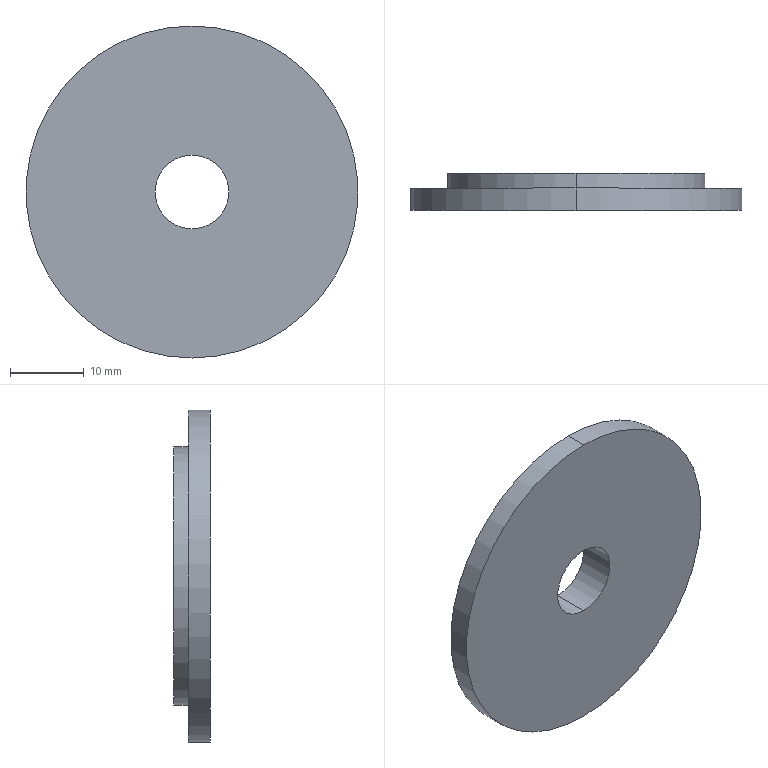Part | SolidWorks | features ICE 2, Extrusion 1 | 1 solid | 9 faces | box 45 x 5 x 45 mm | volume 6303 mm3 | cylinder 6 | plane 3 | commonest cylinder face diameters 10 x2 35 x2 45 x2
STEP:
#1=CARTESIAN_POINT('',(0.,0.,-5.));
#2=VERTEX_POINT('',#1);
#3=CARTESIAN_POINT('',(0.,0.,5.));
#4=VERTEX_POINT('',#3);
#5=CARTESIAN_POINT('',(0.,0.,0.));
#6=DIRECTION('',(0.,1.,0.));
#7=DIRECTION('',(0.,0.,1.));
#8=AXIS2_PLACEMENT_3D('',#5,#6,#7);
#9=CIRCLE('',#8,5.);
#10=EDGE_CURVE('',#2,#4,#9,.T.);
#11=ORIENTED_EDGE('',*,*,#10,.F.);
#12=CARTESIAN_POINT('',(0.,5.,-5.));
#13=VERTEX_POINT('',#12);
#14=CARTESIAN_POINT('',(0.,0.,-5.));
#15=DIRECTION('',(0.,1.,0.));
#16=VECTOR('',#15,1000.);
#17=LINE('',#14,#16);
#18=EDGE_CURVE('',#2,#13,#17,.T.);
#19=ORIENTED_EDGE('',*,*,#18,.T.);
#20=CARTESIAN_POINT('',(0.,5.,5.));
#21=VERTEX_POINT('',#20);
#22=CARTESIAN_POINT('',(0.,5.,0.));
#23=DIRECTION('',(0.,1.,0.));
#24=DIRECTION('',(0.,0.,1.));
#25=AXIS2_PLACEMENT_3D('',#22,#23,#24);
#26=CIRCLE('',#25,5.);
#27=EDGE_CURVE('',#13,#21,#26,.T.);
#28=ORIENTED_EDGE('',*,*,#27,.T.);
#29=CARTESIAN_POINT('',(0.,0.,5.));
#30=DIRECTION('',(0.,1.,0.));
#31=VECTOR('',#30,1000.);
#32=LINE('',#29,#31);
#33=EDGE_CURVE('',#4,#21,#32,.T.);
#34=ORIENTED_EDGE('',*,*,#33,.F.);
#35=EDGE_LOOP('',(#11,#19,#28,#34));
#36=FACE_OUTER_BOUND('',#35,.T.);
#37=CARTESIAN_POINT('',(0.,0.,0.));
#38=DIRECTION('',(0.,1.,0.));
#39=DIRECTION('',(0.,0.,1.));
#40=AXIS2_PLACEMENT_3D('',#37,#38,#39);
#41=CYLINDRICAL_SURFACE('',#40,5.);
#42=ADVANCED_FACE('',(#36),#41,.F.);
#43=CARTESIAN_POINT('',(0.,5.,17.5));
#44=VERTEX_POINT('',#43);
#45=CARTESIAN_POINT('',(0.,5.,-17.5));
#46=VERTEX_POINT('',#45);
#47=CARTESIAN_POINT('',(0.,5.,0.));
#48=DIRECTION('',(0.,1.,0.));
#49=DIRECTION('',(0.,0.,1.));
#50=AXIS2_PLACEMENT_3D('',#47,#48,#49);
#51=CIRCLE('',#50,17.5);
#52=EDGE_CURVE('',#44,#46,#51,.T.);
#53=ORIENTED_EDGE('',*,*,#52,.F.);
#54=CARTESIAN_POINT('',(0.,3.,17.5));
#55=VERTEX_POINT('',#54);
#56=CARTESIAN_POINT('',(0.,5.,17.5));
#57=DIRECTION('',(0.,-1.,0.));
#58=VECTOR('',#57,1000.);
#59=LINE('',#56,#58);
#60=EDGE_CURVE('',#44,#55,#59,.T.);
#61=ORIENTED_EDGE('',*,*,#60,.T.);
#62=CARTESIAN_POINT('',(0.,3.,-17.5));
#63=VERTEX_POINT('',#62);
#64=CARTESIAN_POINT('',(0.,3.,0.));
#65=DIRECTION('',(0.,1.,0.));
#66=DIRECTION('',(0.,0.,1.));
#67=AXIS2_PLACEMENT_3D('',#64,#65,#66);
#68=CIRCLE('',#67,17.5);
#69=EDGE_CURVE('',#55,#63,#68,.T.);
#70=ORIENTED_EDGE('',*,*,#69,.T.);
#71=CARTESIAN_POINT('',(0.,5.,-17.5));
#72=DIRECTION('',(0.,-1.,0.));
#73=VECTOR('',#72,1000.);
#74=LINE('',#71,#73);
#75=EDGE_CURVE('',#46,#63,#74,.T.);
#76=ORIENTED_EDGE('',*,*,#75,.F.);
#77=EDGE_LOOP('',(#53,#61,#70,#76));
#78=FACE_OUTER_BOUND('',#77,.T.);
#79=CARTESIAN_POINT('',(0.,5.,0.));
#80=DIRECTION('',(0.,-1.,0.));
#81=DIRECTION('',(0.,0.,-1.));
#82=AXIS2_PLACEMENT_3D('',#79,#80,#81);
#83=CYLINDRICAL_SURFACE('',#82,17.5);
#84=ADVANCED_FACE('',(#78),#83,.T.);
#85=CARTESIAN_POINT('',(0.,3.,22.5));
#86=VERTEX_POINT('',#85);
#87=CARTESIAN_POINT('',(0.,3.,-22.5));
#88=VERTEX_POINT('',#87);
#89=CARTESIAN_POINT('',(0.,3.,0.));
#90=DIRECTION('',(0.,1.,0.));
#91=DIRECTION('',(0.,0.,1.));
#92=AXIS2_PLACEMENT_3D('',#89,#90,#91);
#93=CIRCLE('',#92,22.5);
#94=EDGE_CURVE('',#86,#88,#93,.T.);
#95=ORIENTED_EDGE('',*,*,#94,.F.);
#96=CARTESIAN_POINT('',(0.,0.,22.5));
#97=VERTEX_POINT('',#96);
#98=CARTESIAN_POINT('',(0.,3.,22.5));
#99=DIRECTION('',(0.,-1.,0.));
#100=VECTOR('',#99,1000.);
#101=LINE('',#98,#100);
#102=EDGE_CURVE('',#86,#97,#101,.T.);
#103=ORIENTED_EDGE('',*,*,#102,.T.);
#104=CARTESIAN_POINT('',(0.,0.,-22.5));
#105=VERTEX_POINT('',#104);
#106=CARTESIAN_POINT('',(0.,0.,0.));
#107=DIRECTION('',(0.,1.,0.));
#108=DIRECTION('',(0.,0.,1.));
#109=AXIS2_PLACEMENT_3D('',#106,#107,#108);
#110=CIRCLE('',#109,22.5);
#111=EDGE_CURVE('',#97,#105,#110,.T.);
#112=ORIENTED_EDGE('',*,*,#111,.T.);
#113=CARTESIAN_POINT('',(0.,3.,-22.5));
#114=DIRECTION('',(0.,-1.,0.));
#115=VECTOR('',#114,1000.);
#116=LINE('',#113,#115);
#117=EDGE_CURVE('',#88,#105,#116,.T.);
#118=ORIENTED_EDGE('',*,*,#117,.F.);
#119=EDGE_LOOP('',(#95,#103,#112,#118));
#120=FACE_OUTER_BOUND('',#119,.T.);
#121=CARTESIAN_POINT('',(0.,3.,0.));
#122=DIRECTION('',(0.,-1.,0.));
#123=DIRECTION('',(0.,0.,-1.));
#124=AXIS2_PLACEMENT_3D('',#121,#122,#123);
#125=CYLINDRICAL_SURFACE('',#124,22.5);
#126=ADVANCED_FACE('',(#120),#125,.T.);
#127=CARTESIAN_POINT('',(0.,3.,0.));
#128=DIRECTION('',(0.,1.,0.));
#129=DIRECTION('',(0.,0.,1.));
#130=AXIS2_PLACEMENT_3D('',#127,#128,#129);
#131=CIRCLE('',#130,22.5);
#132=EDGE_CURVE('',#88,#86,#131,.T.);
#133=ORIENTED_EDGE('',*,*,#132,.T.);
#134=ORIENTED_EDGE('',*,*,#94,.T.);
#135=EDGE_LOOP('',(#133,#134));
#136=FACE_OUTER_BOUND('',#135,.T.);
#137=CARTESIAN_POINT('',(0.,3.,0.));
#138=DIRECTION('',(0.,1.,0.));
#139=DIRECTION('',(0.,0.,1.));
#140=AXIS2_PLACEMENT_3D('',#137,#138,#139);
#141=CIRCLE('',#140,17.5);
#142=EDGE_CURVE('',#63,#55,#141,.T.);
#143=ORIENTED_EDGE('',*,*,#142,.F.);
#144=ORIENTED_EDGE('',*,*,#69,.F.);
#145=EDGE_LOOP('',(#143,#144));
#146=FACE_BOUND('',#145,.T.);
#147=CARTESIAN_POINT('',(0.,3.,0.));
#148=DIRECTION('',(0.,1.,0.));
#149=DIRECTION('',(0.,0.,1.));
#150=AXIS2_PLACEMENT_3D('',#147,#148,#149);
#151=PLANE('',#150);
#152=ADVANCED_FACE('',(#136,#146),#151,.T.);
#153=ORIENTED_EDGE('',*,*,#102,.F.);
#154=ORIENTED_EDGE('',*,*,#132,.F.);
#155=ORIENTED_EDGE('',*,*,#117,.T.);
#156=CARTESIAN_POINT('',(0.,0.,0.));
#157=DIRECTION('',(0.,1.,0.));
#158=DIRECTION('',(0.,0.,1.));
#159=AXIS2_PLACEMENT_3D('',#156,#157,#158);
#160=CIRCLE('',#159,22.5);
#161=EDGE_CURVE('',#105,#97,#160,.T.);
#162=ORIENTED_EDGE('',*,*,#161,.T.);
#163=EDGE_LOOP('',(#153,#154,#155,#162));
#164=FACE_OUTER_BOUND('',#163,.T.);
#165=CARTESIAN_POINT('',(0.,3.,0.));
#166=DIRECTION('',(0.,-1.,0.));
#167=DIRECTION('',(0.,0.,-1.));
#168=AXIS2_PLACEMENT_3D('',#165,#166,#167);
#169=CYLINDRICAL_SURFACE('',#168,22.5);
#170=ADVANCED_FACE('',(#164),#169,.T.);
#171=CARTESIAN_POINT('',(0.,0.,0.));
#172=DIRECTION('',(0.,1.,0.));
#173=DIRECTION('',(0.,0.,1.));
#174=AXIS2_PLACEMENT_3D('',#171,#172,#173);
#175=CIRCLE('',#174,5.);
#176=EDGE_CURVE('',#4,#2,#175,.T.);
#177=ORIENTED_EDGE('',*,*,#176,.T.);
#178=ORIENTED_EDGE('',*,*,#10,.T.);
#179=EDGE_LOOP('',(#177,#178));
#180=FACE_BOUND('',#179,.T.);
#181=ORIENTED_EDGE('',*,*,#161,.F.);
#182=ORIENTED_EDGE('',*,*,#111,.F.);
#183=EDGE_LOOP('',(#181,#182));
#184=FACE_OUTER_BOUND('',#183,.T.);
#185=CARTESIAN_POINT('',(0.,0.,0.));
#186=DIRECTION('',(0.,1.,0.));
#187=DIRECTION('',(0.,0.,1.));
#188=AXIS2_PLACEMENT_3D('',#185,#186,#187);
#189=PLANE('',#188);
#190=ADVANCED_FACE('',(#180,#184),#189,.F.);
#191=ORIENTED_EDGE('',*,*,#60,.F.);
#192=CARTESIAN_POINT('',(0.,5.,0.));
#193=DIRECTION('',(0.,1.,0.));
#194=DIRECTION('',(0.,0.,1.));
#195=AXIS2_PLACEMENT_3D('',#192,#193,#194);
#196=CIRCLE('',#195,17.5);
#197=EDGE_CURVE('',#46,#44,#196,.T.);
#198=ORIENTED_EDGE('',*,*,#197,.F.);
#199=ORIENTED_EDGE('',*,*,#75,.T.);
#200=ORIENTED_EDGE('',*,*,#142,.T.);
#201=EDGE_LOOP('',(#191,#198,#199,#200));
#202=FACE_OUTER_BOUND('',#201,.T.);
#203=CARTESIAN_POINT('',(0.,5.,0.));
#204=DIRECTION('',(0.,-1.,0.));
#205=DIRECTION('',(0.,0.,-1.));
#206=AXIS2_PLACEMENT_3D('',#203,#204,#205);
#207=CYLINDRICAL_SURFACE('',#206,17.5);
#208=ADVANCED_FACE('',(#202),#207,.T.);
#209=CARTESIAN_POINT('',(0.,5.,0.));
#210=DIRECTION('',(0.,1.,0.));
#211=DIRECTION('',(0.,0.,1.));
#212=AXIS2_PLACEMENT_3D('',#209,#210,#211);
#213=CIRCLE('',#212,5.);
#214=EDGE_CURVE('',#21,#13,#213,.T.);
#215=ORIENTED_EDGE('',*,*,#214,.F.);
#216=ORIENTED_EDGE('',*,*,#27,.F.);
#217=EDGE_LOOP('',(#215,#216));
#218=FACE_BOUND('',#217,.T.);
#219=ORIENTED_EDGE('',*,*,#197,.T.);
#220=ORIENTED_EDGE('',*,*,#52,.T.);
#221=EDGE_LOOP('',(#219,#220));
#222=FACE_OUTER_BOUND('',#221,.T.);
#223=CARTESIAN_POINT('',(0.,5.,0.));
#224=DIRECTION('',(0.,1.,0.));
#225=DIRECTION('',(0.,0.,1.));
#226=AXIS2_PLACEMENT_3D('',#223,#224,#225);
#227=PLANE('',#226);
#228=ADVANCED_FACE('',(#218,#222),#227,.T.);
#229=ORIENTED_EDGE('',*,*,#18,.F.);
#230=ORIENTED_EDGE('',*,*,#176,.F.);
#231=ORIENTED_EDGE('',*,*,#33,.T.);
#232=ORIENTED_EDGE('',*,*,#214,.T.);
#233=EDGE_LOOP('',(#229,#230,#231,#232));
#234=FACE_OUTER_BOUND('',#233,.T.);
#235=CARTESIAN_POINT('',(0.,0.,0.));
#236=DIRECTION('',(0.,1.,0.));
#237=DIRECTION('',(0.,0.,1.));
#238=AXIS2_PLACEMENT_3D('',#235,#236,#237);
#239=CYLINDRICAL_SURFACE('',#238,5.);
#240=ADVANCED_FACE('',(#234),#239,.F.);
#241=CLOSED_SHELL('',(#42,#84,#126,#152,#170,#190,#208,#228,#240));
#242=MANIFOLD_SOLID_BREP('',#241);
#243=CARTESIAN_POINT('',(0.,0.,0.));
#244=DIRECTION('',(0.,0.,1.));
#245=DIRECTION('',(1.,0.,0.));
#246=AXIS2_PLACEMENT_3D('',#243,#244,#245);
#247=(LENGTH_UNIT()NAMED_UNIT(*)SI_UNIT(.MILLI.,.METRE.));
#248=UNCERTAINTY_MEASURE_WITH_UNIT(LENGTH_MEASURE(0.00001),#247,'','');
#249=(NAMED_UNIT(*)PLANE_ANGLE_UNIT()SI_UNIT($,.RADIAN.));
#250=(NAMED_UNIT(*)SI_UNIT($,.STERADIAN.)SOLID_ANGLE_UNIT());
#251=(GEOMETRIC_REPRESENTATION_CONTEXT(3)GLOBAL_UNCERTAINTY_ASSIGNED_CONTEXT((#248))GLOBAL_UNIT_ASSIGNED_CONTEXT((#247,#249,#250))REPRESENTATION_CONTEXT('',''));
#252=ADVANCED_BREP_SHAPE_REPRESENTATION('',(#242,#246),#251);